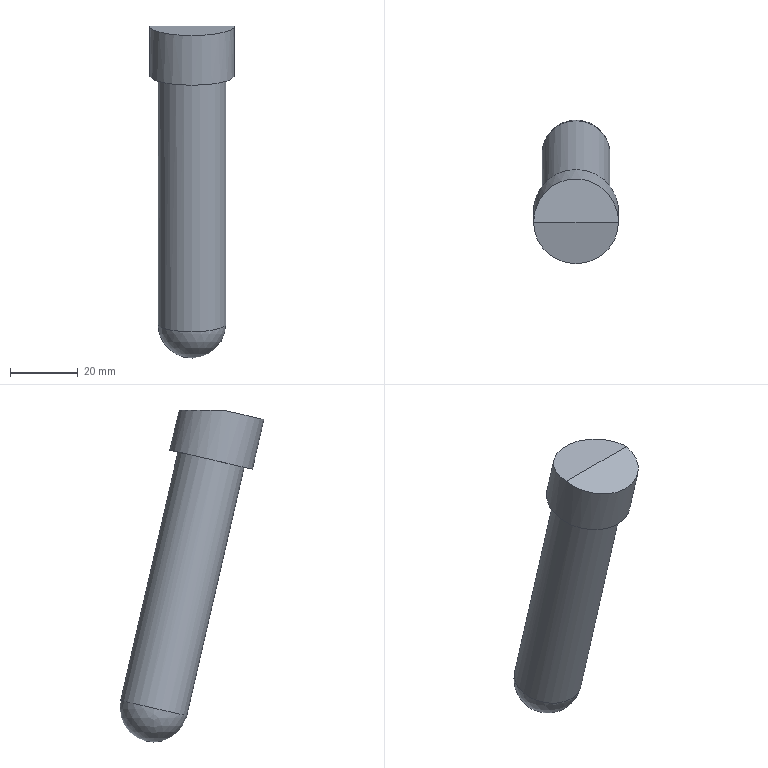Part | STEP file | solid 1 | 1 solid | 6 faces | box 25 x 42.455 x 97.821 mm | volume 32760 mm3 | plane 3 | cylinder 2 | sphere 1 | commonest cylinder face diameters 20 x1 25 x1